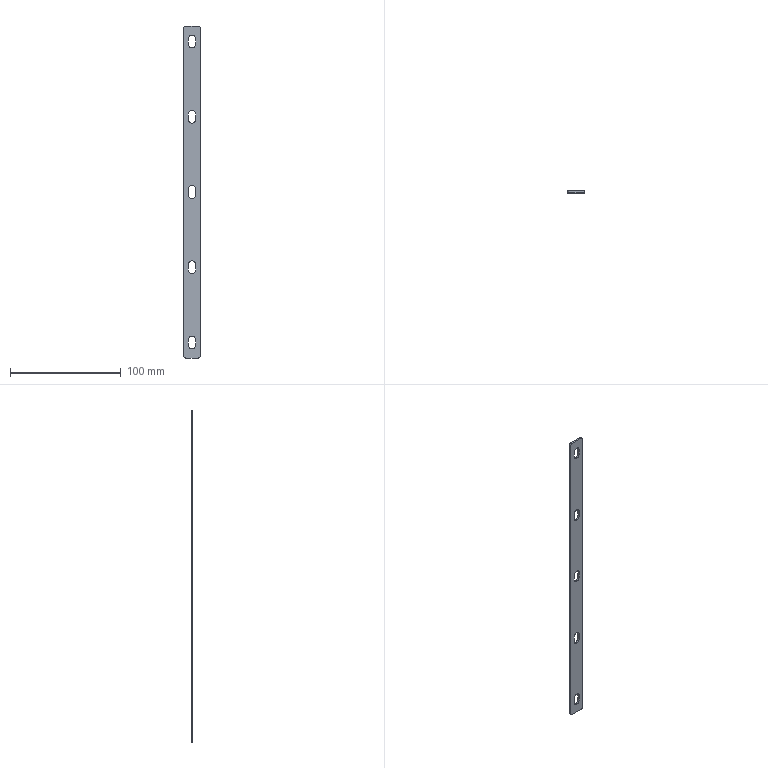Part | 1 solid | 35 faces | box 15 x 1.5 x 300 mm | volume 6252 mm3 | cylinder 19 | plane 16 | commonest cylinder face diameters 6.5 x15 4 x4
STEP:
#1=CARTESIAN_POINT('',(0.,-1.5,141.75));
#2=VERTEX_POINT('',#1);
#3=CARTESIAN_POINT('',(3.25,-1.5,138.5));
#4=VERTEX_POINT('',#3);
#5=CARTESIAN_POINT('',(0.,-1.5,138.5));
#6=DIRECTION('',(0.,1.,0.));
#7=DIRECTION('',(0.,0.,1.));
#8=AXIS2_PLACEMENT_3D('',#5,#6,#7);
#9=CIRCLE('',#8,3.25);
#10=EDGE_CURVE('',#2,#4,#9,.T.);
#11=ORIENTED_EDGE('',*,*,#10,.F.);
#12=CARTESIAN_POINT('',(0.,0.,141.75));
#13=VERTEX_POINT('',#12);
#14=CARTESIAN_POINT('',(0.,-1.5,141.75));
#15=DIRECTION('',(0.,1.,0.));
#16=VECTOR('',#15,1000.);
#17=LINE('',#14,#16);
#18=EDGE_CURVE('',#2,#13,#17,.T.);
#19=ORIENTED_EDGE('',*,*,#18,.T.);
#20=CARTESIAN_POINT('',(3.25,0.,138.5));
#21=VERTEX_POINT('',#20);
#22=CARTESIAN_POINT('',(0.,0.,138.5));
#23=DIRECTION('',(0.,1.,0.));
#24=DIRECTION('',(0.,0.,1.));
#25=AXIS2_PLACEMENT_3D('',#22,#23,#24);
#26=CIRCLE('',#25,3.25);
#27=EDGE_CURVE('',#13,#21,#26,.T.);
#28=ORIENTED_EDGE('',*,*,#27,.T.);
#29=CARTESIAN_POINT('',(3.25,-1.5,138.5));
#30=DIRECTION('',(0.,1.,0.));
#31=VECTOR('',#30,1000.);
#32=LINE('',#29,#31);
#33=EDGE_CURVE('',#4,#21,#32,.T.);
#34=ORIENTED_EDGE('',*,*,#33,.F.);
#35=EDGE_LOOP('',(#11,#19,#28,#34));
#36=FACE_OUTER_BOUND('',#35,.T.);
#37=CARTESIAN_POINT('',(0.,-1.5,138.5));
#38=DIRECTION('',(0.,1.,0.));
#39=DIRECTION('',(0.,0.,1.));
#40=AXIS2_PLACEMENT_3D('',#37,#38,#39);
#41=CYLINDRICAL_SURFACE('',#40,3.25);
#42=ADVANCED_FACE('',(#36),#41,.F.);
#43=CARTESIAN_POINT('',(0.,-1.5,73.75));
#44=VERTEX_POINT('',#43);
#45=CARTESIAN_POINT('',(3.25,-1.5,70.5));
#46=VERTEX_POINT('',#45);
#47=CARTESIAN_POINT('',(0.,-1.5,70.5));
#48=DIRECTION('',(0.,1.,0.));
#49=DIRECTION('',(0.,0.,1.));
#50=AXIS2_PLACEMENT_3D('',#47,#48,#49);
#51=CIRCLE('',#50,3.25);
#52=EDGE_CURVE('',#44,#46,#51,.T.);
#53=ORIENTED_EDGE('',*,*,#52,.F.);
#54=CARTESIAN_POINT('',(0.,0.,73.75));
#55=VERTEX_POINT('',#54);
#56=CARTESIAN_POINT('',(0.,-1.5,73.75));
#57=DIRECTION('',(0.,1.,0.));
#58=VECTOR('',#57,1000.);
#59=LINE('',#56,#58);
#60=EDGE_CURVE('',#44,#55,#59,.T.);
#61=ORIENTED_EDGE('',*,*,#60,.T.);
#62=CARTESIAN_POINT('',(3.25,0.,70.5));
#63=VERTEX_POINT('',#62);
#64=CARTESIAN_POINT('',(0.,0.,70.5));
#65=DIRECTION('',(0.,1.,0.));
#66=DIRECTION('',(0.,0.,1.));
#67=AXIS2_PLACEMENT_3D('',#64,#65,#66);
#68=CIRCLE('',#67,3.25);
#69=EDGE_CURVE('',#55,#63,#68,.T.);
#70=ORIENTED_EDGE('',*,*,#69,.T.);
#71=CARTESIAN_POINT('',(3.25,-1.5,70.5));
#72=DIRECTION('',(0.,1.,0.));
#73=VECTOR('',#72,1000.);
#74=LINE('',#71,#73);
#75=EDGE_CURVE('',#46,#63,#74,.T.);
#76=ORIENTED_EDGE('',*,*,#75,.F.);
#77=EDGE_LOOP('',(#53,#61,#70,#76));
#78=FACE_OUTER_BOUND('',#77,.T.);
#79=CARTESIAN_POINT('',(0.,-1.5,70.5));
#80=DIRECTION('',(0.,1.,0.));
#81=DIRECTION('',(0.,0.,1.));
#82=AXIS2_PLACEMENT_3D('',#79,#80,#81);
#83=CYLINDRICAL_SURFACE('',#82,3.25);
#84=ADVANCED_FACE('',(#78),#83,.F.);
#85=CARTESIAN_POINT('',(0.,-1.5,5.75));
#86=VERTEX_POINT('',#85);
#87=CARTESIAN_POINT('',(3.25,-1.5,2.5));
#88=VERTEX_POINT('',#87);
#89=CARTESIAN_POINT('',(0.,-1.5,2.5));
#90=DIRECTION('',(0.,1.,0.));
#91=DIRECTION('',(0.,0.,1.));
#92=AXIS2_PLACEMENT_3D('',#89,#90,#91);
#93=CIRCLE('',#92,3.25);
#94=EDGE_CURVE('',#86,#88,#93,.T.);
#95=ORIENTED_EDGE('',*,*,#94,.F.);
#96=CARTESIAN_POINT('',(0.,0.,5.75));
#97=VERTEX_POINT('',#96);
#98=CARTESIAN_POINT('',(0.,-1.5,5.75));
#99=DIRECTION('',(0.,1.,0.));
#100=VECTOR('',#99,1000.);
#101=LINE('',#98,#100);
#102=EDGE_CURVE('',#86,#97,#101,.T.);
#103=ORIENTED_EDGE('',*,*,#102,.T.);
#104=CARTESIAN_POINT('',(3.25,0.,2.5));
#105=VERTEX_POINT('',#104);
#106=CARTESIAN_POINT('',(0.,0.,2.5));
#107=DIRECTION('',(0.,1.,0.));
#108=DIRECTION('',(0.,0.,1.));
#109=AXIS2_PLACEMENT_3D('',#106,#107,#108);
#110=CIRCLE('',#109,3.25);
#111=EDGE_CURVE('',#97,#105,#110,.T.);
#112=ORIENTED_EDGE('',*,*,#111,.T.);
#113=CARTESIAN_POINT('',(3.25,-1.5,2.5));
#114=DIRECTION('',(0.,1.,0.));
#115=VECTOR('',#114,1000.);
#116=LINE('',#113,#115);
#117=EDGE_CURVE('',#88,#105,#116,.T.);
#118=ORIENTED_EDGE('',*,*,#117,.F.);
#119=EDGE_LOOP('',(#95,#103,#112,#118));
#120=FACE_OUTER_BOUND('',#119,.T.);
#121=CARTESIAN_POINT('',(0.,-1.5,2.5));
#122=DIRECTION('',(0.,1.,0.));
#123=DIRECTION('',(0.,0.,1.));
#124=AXIS2_PLACEMENT_3D('',#121,#122,#123);
#125=CYLINDRICAL_SURFACE('',#124,3.25);
#126=ADVANCED_FACE('',(#120),#125,.F.);
#127=CARTESIAN_POINT('',(0.,-1.5,-62.25));
#128=VERTEX_POINT('',#127);
#129=CARTESIAN_POINT('',(3.25,-1.5,-65.5));
#130=VERTEX_POINT('',#129);
#131=CARTESIAN_POINT('',(0.,-1.5,-65.5));
#132=DIRECTION('',(0.,1.,0.));
#133=DIRECTION('',(0.,0.,1.));
#134=AXIS2_PLACEMENT_3D('',#131,#132,#133);
#135=CIRCLE('',#134,3.25);
#136=EDGE_CURVE('',#128,#130,#135,.T.);
#137=ORIENTED_EDGE('',*,*,#136,.F.);
#138=CARTESIAN_POINT('',(0.,0.,-62.25));
#139=VERTEX_POINT('',#138);
#140=CARTESIAN_POINT('',(0.,-1.5,-62.25));
#141=DIRECTION('',(0.,1.,0.));
#142=VECTOR('',#141,1000.);
#143=LINE('',#140,#142);
#144=EDGE_CURVE('',#128,#139,#143,.T.);
#145=ORIENTED_EDGE('',*,*,#144,.T.);
#146=CARTESIAN_POINT('',(3.25,0.,-65.5));
#147=VERTEX_POINT('',#146);
#148=CARTESIAN_POINT('',(0.,0.,-65.5));
#149=DIRECTION('',(0.,1.,0.));
#150=DIRECTION('',(0.,0.,1.));
#151=AXIS2_PLACEMENT_3D('',#148,#149,#150);
#152=CIRCLE('',#151,3.25);
#153=EDGE_CURVE('',#139,#147,#152,.T.);
#154=ORIENTED_EDGE('',*,*,#153,.T.);
#155=CARTESIAN_POINT('',(3.25,-1.5,-65.5));
#156=DIRECTION('',(0.,1.,0.));
#157=VECTOR('',#156,1000.);
#158=LINE('',#155,#157);
#159=EDGE_CURVE('',#130,#147,#158,.T.);
#160=ORIENTED_EDGE('',*,*,#159,.F.);
#161=EDGE_LOOP('',(#137,#145,#154,#160));
#162=FACE_OUTER_BOUND('',#161,.T.);
#163=CARTESIAN_POINT('',(0.,-1.5,-65.5));
#164=DIRECTION('',(0.,1.,0.));
#165=DIRECTION('',(0.,0.,1.));
#166=AXIS2_PLACEMENT_3D('',#163,#164,#165);
#167=CYLINDRICAL_SURFACE('',#166,3.25);
#168=ADVANCED_FACE('',(#162),#167,.F.);
#169=CARTESIAN_POINT('',(0.,-1.5,-130.25));
#170=VERTEX_POINT('',#169);
#171=CARTESIAN_POINT('',(3.25,-1.5,-133.5));
#172=VERTEX_POINT('',#171);
#173=CARTESIAN_POINT('',(0.,-1.5,-133.5));
#174=DIRECTION('',(0.,1.,0.));
#175=DIRECTION('',(0.,0.,1.));
#176=AXIS2_PLACEMENT_3D('',#173,#174,#175);
#177=CIRCLE('',#176,3.25);
#178=EDGE_CURVE('',#170,#172,#177,.T.);
#179=ORIENTED_EDGE('',*,*,#178,.F.);
#180=CARTESIAN_POINT('',(0.,0.,-130.25));
#181=VERTEX_POINT('',#180);
#182=CARTESIAN_POINT('',(0.,-1.5,-130.25));
#183=DIRECTION('',(0.,1.,0.));
#184=VECTOR('',#183,1000.);
#185=LINE('',#182,#184);
#186=EDGE_CURVE('',#170,#181,#185,.T.);
#187=ORIENTED_EDGE('',*,*,#186,.T.);
#188=CARTESIAN_POINT('',(3.25,0.,-133.5));
#189=VERTEX_POINT('',#188);
#190=CARTESIAN_POINT('',(0.,0.,-133.5));
#191=DIRECTION('',(0.,1.,0.));
#192=DIRECTION('',(0.,0.,1.));
#193=AXIS2_PLACEMENT_3D('',#190,#191,#192);
#194=CIRCLE('',#193,3.25);
#195=EDGE_CURVE('',#181,#189,#194,.T.);
#196=ORIENTED_EDGE('',*,*,#195,.T.);
#197=CARTESIAN_POINT('',(3.25,-1.5,-133.5));
#198=DIRECTION('',(0.,1.,0.));
#199=VECTOR('',#198,1000.);
#200=LINE('',#197,#199);
#201=EDGE_CURVE('',#172,#189,#200,.T.);
#202=ORIENTED_EDGE('',*,*,#201,.F.);
#203=EDGE_LOOP('',(#179,#187,#196,#202));
#204=FACE_OUTER_BOUND('',#203,.T.);
#205=CARTESIAN_POINT('',(0.,-1.5,-133.5));
#206=DIRECTION('',(0.,1.,0.));
#207=DIRECTION('',(0.,0.,1.));
#208=AXIS2_PLACEMENT_3D('',#205,#206,#207);
#209=CYLINDRICAL_SURFACE('',#208,3.25);
#210=ADVANCED_FACE('',(#204),#209,.F.);
#211=CARTESIAN_POINT('',(7.5,0.,148.));
#212=VERTEX_POINT('',#211);
#213=CARTESIAN_POINT('',(7.5,0.,-148.));
#214=VERTEX_POINT('',#213);
#215=CARTESIAN_POINT('',(7.5,0.,150.));
#216=DIRECTION('',(0.,0.,-1.));
#217=VECTOR('',#216,1000.);
#218=LINE('',#215,#217);
#219=EDGE_CURVE('',#212,#214,#218,.T.);
#220=ORIENTED_EDGE('',*,*,#219,.F.);
#221=CARTESIAN_POINT('',(7.5,-1.5,148.));
#222=VERTEX_POINT('',#221);
#223=CARTESIAN_POINT('',(7.5,-1.5,148.));
#224=DIRECTION('',(0.,-1.,0.));
#225=VECTOR('',#224,1000.);
#226=LINE('',#223,#225);
#227=EDGE_CURVE('',#212,#222,#226,.T.);
#228=ORIENTED_EDGE('',*,*,#227,.T.);
#229=CARTESIAN_POINT('',(7.5,-1.5,-148.));
#230=VERTEX_POINT('',#229);
#231=CARTESIAN_POINT('',(7.5,-1.5,150.));
#232=DIRECTION('',(0.,0.,-1.));
#233=VECTOR('',#232,1000.);
#234=LINE('',#231,#233);
#235=EDGE_CURVE('',#222,#230,#234,.T.);
#236=ORIENTED_EDGE('',*,*,#235,.T.);
#237=CARTESIAN_POINT('',(7.5,-1.5,-148.));
#238=DIRECTION('',(0.,1.,0.));
#239=VECTOR('',#238,1000.);
#240=LINE('',#237,#239);
#241=EDGE_CURVE('',#230,#214,#240,.T.);
#242=ORIENTED_EDGE('',*,*,#241,.T.);
#243=EDGE_LOOP('',(#220,#228,#236,#242));
#244=FACE_OUTER_BOUND('',#243,.T.);
#245=CARTESIAN_POINT('',(7.5,-1.5,150.));
#246=DIRECTION('',(1.,0.,0.));
#247=DIRECTION('',(0.,0.,-1.));
#248=AXIS2_PLACEMENT_3D('',#245,#246,#247);
#249=PLANE('',#248);
#250=ADVANCED_FACE('',(#244),#249,.T.);
#251=CARTESIAN_POINT('',(-5.5,-1.5,150.));
#252=VERTEX_POINT('',#251);
#253=CARTESIAN_POINT('',(5.5,-1.5,150.));
#254=VERTEX_POINT('',#253);
#255=CARTESIAN_POINT('',(-7.5,-1.5,150.));
#256=DIRECTION('',(1.,0.,0.));
#257=VECTOR('',#256,1000.);
#258=LINE('',#255,#257);
#259=EDGE_CURVE('',#252,#254,#258,.T.);
#260=ORIENTED_EDGE('',*,*,#259,.T.);
#261=CARTESIAN_POINT('',(5.5,0.,150.));
#262=VERTEX_POINT('',#261);
#263=CARTESIAN_POINT('',(5.5,-1.5,150.));
#264=DIRECTION('',(0.,1.,0.));
#265=VECTOR('',#264,1000.);
#266=LINE('',#263,#265);
#267=EDGE_CURVE('',#254,#262,#266,.T.);
#268=ORIENTED_EDGE('',*,*,#267,.T.);
#269=CARTESIAN_POINT('',(-5.5,0.,150.));
#270=VERTEX_POINT('',#269);
#271=CARTESIAN_POINT('',(-7.5,0.,150.));
#272=DIRECTION('',(1.,0.,0.));
#273=VECTOR('',#272,1000.);
#274=LINE('',#271,#273);
#275=EDGE_CURVE('',#270,#262,#274,.T.);
#276=ORIENTED_EDGE('',*,*,#275,.F.);
#277=CARTESIAN_POINT('',(-5.5,-1.5,150.));
#278=DIRECTION('',(0.,-1.,0.));
#279=VECTOR('',#278,1000.);
#280=LINE('',#277,#279);
#281=EDGE_CURVE('',#270,#252,#280,.T.);
#282=ORIENTED_EDGE('',*,*,#281,.T.);
#283=EDGE_LOOP('',(#260,#268,#276,#282));
#284=FACE_OUTER_BOUND('',#283,.T.);
#285=CARTESIAN_POINT('',(-7.5,-1.5,150.));
#286=DIRECTION('',(0.,0.,1.));
#287=DIRECTION('',(1.,0.,0.));
#288=AXIS2_PLACEMENT_3D('',#285,#286,#287);
#289=PLANE('',#288);
#290=ADVANCED_FACE('',(#284),#289,.T.);
#291=CARTESIAN_POINT('',(-7.5,-1.5,-148.));
#292=VERTEX_POINT('',#291);
#293=CARTESIAN_POINT('',(-7.5,-1.5,148.));
#294=VERTEX_POINT('',#293);
#295=CARTESIAN_POINT('',(-7.5,-1.5,150.));
#296=DIRECTION('',(0.,0.,1.));
#297=VECTOR('',#296,1000.);
#298=LINE('',#295,#297);
#299=EDGE_CURVE('',#292,#294,#298,.T.);
#300=ORIENTED_EDGE('',*,*,#299,.T.);
#301=CARTESIAN_POINT('',(-7.5,0.,148.));
#302=VERTEX_POINT('',#301);
#303=CARTESIAN_POINT('',(-7.5,-1.5,148.));
#304=DIRECTION('',(0.,1.,0.));
#305=VECTOR('',#304,1000.);
#306=LINE('',#303,#305);
#307=EDGE_CURVE('',#294,#302,#306,.T.);
#308=ORIENTED_EDGE('',*,*,#307,.T.);
#309=CARTESIAN_POINT('',(-7.5,0.,-148.));
#310=VERTEX_POINT('',#309);
#311=CARTESIAN_POINT('',(-7.5,0.,150.));
#312=DIRECTION('',(0.,0.,1.));
#313=VECTOR('',#312,1000.);
#314=LINE('',#311,#313);
#315=EDGE_CURVE('',#310,#302,#314,.T.);
#316=ORIENTED_EDGE('',*,*,#315,.F.);
#317=CARTESIAN_POINT('',(-7.5,-1.5,-148.));
#318=DIRECTION('',(0.,-1.,0.));
#319=VECTOR('',#318,1000.);
#320=LINE('',#317,#319);
#321=EDGE_CURVE('',#310,#292,#320,.T.);
#322=ORIENTED_EDGE('',*,*,#321,.T.);
#323=EDGE_LOOP('',(#300,#308,#316,#322));
#324=FACE_OUTER_BOUND('',#323,.T.);
#325=CARTESIAN_POINT('',(-7.5,-1.5,150.));
#326=DIRECTION('',(-1.,0.,0.));
#327=DIRECTION('',(0.,0.,1.));
#328=AXIS2_PLACEMENT_3D('',#325,#326,#327);
#329=PLANE('',#328);
#330=ADVANCED_FACE('',(#324),#329,.T.);
#331=CARTESIAN_POINT('',(5.5,-1.5,-150.));
#332=VERTEX_POINT('',#331);
#333=CARTESIAN_POINT('',(-5.5,-1.5,-150.));
#334=VERTEX_POINT('',#333);
#335=CARTESIAN_POINT('',(-7.5,-1.5,-150.));
#336=DIRECTION('',(-1.,0.,0.));
#337=VECTOR('',#336,1000.);
#338=LINE('',#335,#337);
#339=EDGE_CURVE('',#332,#334,#338,.T.);
#340=ORIENTED_EDGE('',*,*,#339,.T.);
#341=CARTESIAN_POINT('',(-5.5,0.,-150.));
#342=VERTEX_POINT('',#341);
#343=CARTESIAN_POINT('',(-5.5,-1.5,-150.));
#344=DIRECTION('',(0.,1.,0.));
#345=VECTOR('',#344,1000.);
#346=LINE('',#343,#345);
#347=EDGE_CURVE('',#334,#342,#346,.T.);
#348=ORIENTED_EDGE('',*,*,#347,.T.);
#349=CARTESIAN_POINT('',(5.5,0.,-150.));
#350=VERTEX_POINT('',#349);
#351=CARTESIAN_POINT('',(-7.5,0.,-150.));
#352=DIRECTION('',(-1.,0.,0.));
#353=VECTOR('',#352,1000.);
#354=LINE('',#351,#353);
#355=EDGE_CURVE('',#350,#342,#354,.T.);
#356=ORIENTED_EDGE('',*,*,#355,.F.);
#357=CARTESIAN_POINT('',(5.5,-1.5,-150.));
#358=DIRECTION('',(0.,-1.,0.));
#359=VECTOR('',#358,1000.);
#360=LINE('',#357,#359);
#361=EDGE_CURVE('',#350,#332,#360,.T.);
#362=ORIENTED_EDGE('',*,*,#361,.T.);
#363=EDGE_LOOP('',(#340,#348,#356,#362));
#364=FACE_OUTER_BOUND('',#363,.T.);
#365=CARTESIAN_POINT('',(-7.5,-1.5,-150.));
#366=DIRECTION('',(0.,0.,-1.));
#367=DIRECTION('',(-1.,0.,0.));
#368=AXIS2_PLACEMENT_3D('',#365,#366,#367);
#369=PLANE('',#368);
#370=ADVANCED_FACE('',(#364),#369,.T.);
#371=CARTESIAN_POINT('',(-3.25,-1.5,138.5));
#372=VERTEX_POINT('',#371);
#373=CARTESIAN_POINT('',(0.,-1.5,138.5));
#374=DIRECTION('',(0.,1.,0.));
#375=DIRECTION('',(0.,0.,1.));
#376=AXIS2_PLACEMENT_3D('',#373,#374,#375);
#377=CIRCLE('',#376,3.25);
#378=EDGE_CURVE('',#372,#2,#377,.T.);
#379=ORIENTED_EDGE('',*,*,#378,.T.);
#380=ORIENTED_EDGE('',*,*,#10,.T.);
#381=CARTESIAN_POINT('',(3.25,-1.5,133.5));
#382=VERTEX_POINT('',#381);
#383=CARTESIAN_POINT('',(3.25,-1.5,138.5));
#384=DIRECTION('',(0.,0.,-1.));
#385=VECTOR('',#384,1000.);
#386=LINE('',#383,#385);
#387=EDGE_CURVE('',#4,#382,#386,.T.);
#388=ORIENTED_EDGE('',*,*,#387,.T.);
#389=CARTESIAN_POINT('',(-3.25,-1.5,133.5));
#390=VERTEX_POINT('',#389);
#391=CARTESIAN_POINT('',(0.,-1.5,133.5));
#392=DIRECTION('',(0.,1.,0.));
#393=DIRECTION('',(0.,0.,1.));
#394=AXIS2_PLACEMENT_3D('',#391,#392,#393);
#395=CIRCLE('',#394,3.25);
#396=EDGE_CURVE('',#382,#390,#395,.T.);
#397=ORIENTED_EDGE('',*,*,#396,.T.);
#398=CARTESIAN_POINT('',(-3.25,-1.5,138.5));
#399=DIRECTION('',(0.,0.,1.));
#400=VECTOR('',#399,1000.);
#401=LINE('',#398,#400);
#402=EDGE_CURVE('',#390,#372,#401,.T.);
#403=ORIENTED_EDGE('',*,*,#402,.T.);
#404=EDGE_LOOP('',(#379,#380,#388,#397,#403));
#405=FACE_BOUND('',#404,.T.);
#406=CARTESIAN_POINT('',(-3.25,-1.5,70.5));
#407=VERTEX_POINT('',#406);
#408=CARTESIAN_POINT('',(0.,-1.5,70.5));
#409=DIRECTION('',(0.,1.,0.));
#410=DIRECTION('',(0.,0.,1.));
#411=AXIS2_PLACEMENT_3D('',#408,#409,#410);
#412=CIRCLE('',#411,3.25);
#413=EDGE_CURVE('',#407,#44,#412,.T.);
#414=ORIENTED_EDGE('',*,*,#413,.T.);
#415=ORIENTED_EDGE('',*,*,#52,.T.);
#416=CARTESIAN_POINT('',(3.25,-1.5,65.5));
#417=VERTEX_POINT('',#416);
#418=CARTESIAN_POINT('',(3.25,-1.5,70.5));
#419=DIRECTION('',(0.,0.,-1.));
#420=VECTOR('',#419,1000.);
#421=LINE('',#418,#420);
#422=EDGE_CURVE('',#46,#417,#421,.T.);
#423=ORIENTED_EDGE('',*,*,#422,.T.);
#424=CARTESIAN_POINT('',(-3.25,-1.5,65.5));
#425=VERTEX_POINT('',#424);
#426=CARTESIAN_POINT('',(0.,-1.5,65.5));
#427=DIRECTION('',(0.,1.,0.));
#428=DIRECTION('',(0.,0.,1.));
#429=AXIS2_PLACEMENT_3D('',#426,#427,#428);
#430=CIRCLE('',#429,3.25);
#431=EDGE_CURVE('',#417,#425,#430,.T.);
#432=ORIENTED_EDGE('',*,*,#431,.T.);
#433=CARTESIAN_POINT('',(-3.25,-1.5,70.5));
#434=DIRECTION('',(0.,0.,1.));
#435=VECTOR('',#434,1000.);
#436=LINE('',#433,#435);
#437=EDGE_CURVE('',#425,#407,#436,.T.);
#438=ORIENTED_EDGE('',*,*,#437,.T.);
#439=EDGE_LOOP('',(#414,#415,#423,#432,#438));
#440=FACE_BOUND('',#439,.T.);
#441=CARTESIAN_POINT('',(-3.25,-1.5,2.5));
#442=VERTEX_POINT('',#441);
#443=CARTESIAN_POINT('',(0.,-1.5,2.5));
#444=DIRECTION('',(0.,1.,0.));
#445=DIRECTION('',(0.,0.,1.));
#446=AXIS2_PLACEMENT_3D('',#443,#444,#445);
#447=CIRCLE('',#446,3.25);
#448=EDGE_CURVE('',#442,#86,#447,.T.);
#449=ORIENTED_EDGE('',*,*,#448,.T.);
#450=ORIENTED_EDGE('',*,*,#94,.T.);
#451=CARTESIAN_POINT('',(3.25,-1.5,-2.5));
#452=VERTEX_POINT('',#451);
#453=CARTESIAN_POINT('',(3.25,-1.5,2.5));
#454=DIRECTION('',(0.,0.,-1.));
#455=VECTOR('',#454,1000.);
#456=LINE('',#453,#455);
#457=EDGE_CURVE('',#88,#452,#456,.T.);
#458=ORIENTED_EDGE('',*,*,#457,.T.);
#459=CARTESIAN_POINT('',(-3.25,-1.5,-2.5));
#460=VERTEX_POINT('',#459);
#461=CARTESIAN_POINT('',(0.,-1.5,-2.5));
#462=DIRECTION('',(0.,1.,0.));
#463=DIRECTION('',(0.,0.,1.));
#464=AXIS2_PLACEMENT_3D('',#461,#462,#463);
#465=CIRCLE('',#464,3.25);
#466=EDGE_CURVE('',#452,#460,#465,.T.);
#467=ORIENTED_EDGE('',*,*,#466,.T.);
#468=CARTESIAN_POINT('',(-3.25,-1.5,2.5));
#469=DIRECTION('',(0.,0.,1.));
#470=VECTOR('',#469,1000.);
#471=LINE('',#468,#470);
#472=EDGE_CURVE('',#460,#442,#471,.T.);
#473=ORIENTED_EDGE('',*,*,#472,.T.);
#474=EDGE_LOOP('',(#449,#450,#458,#467,#473));
#475=FACE_BOUND('',#474,.T.);
#476=CARTESIAN_POINT('',(-3.25,-1.5,-65.5));
#477=VERTEX_POINT('',#476);
#478=CARTESIAN_POINT('',(0.,-1.5,-65.5));
#479=DIRECTION('',(0.,1.,0.));
#480=DIRECTION('',(0.,0.,1.));
#481=AXIS2_PLACEMENT_3D('',#478,#479,#480);
#482=CIRCLE('',#481,3.25);
#483=EDGE_CURVE('',#477,#128,#482,.T.);
#484=ORIENTED_EDGE('',*,*,#483,.T.);
#485=ORIENTED_EDGE('',*,*,#136,.T.);
#486=CARTESIAN_POINT('',(3.25,-1.5,-70.5));
#487=VERTEX_POINT('',#486);
#488=CARTESIAN_POINT('',(3.25,-1.5,-65.5));
#489=DIRECTION('',(0.,0.,-1.));
#490=VECTOR('',#489,1000.);
#491=LINE('',#488,#490);
#492=EDGE_CURVE('',#130,#487,#491,.T.);
#493=ORIENTED_EDGE('',*,*,#492,.T.);
#494=CARTESIAN_POINT('',(-3.25,-1.5,-70.5));
#495=VERTEX_POINT('',#494);
#496=CARTESIAN_POINT('',(0.,-1.5,-70.5));
#497=DIRECTION('',(0.,1.,0.));
#498=DIRECTION('',(0.,0.,1.));
#499=AXIS2_PLACEMENT_3D('',#496,#497,#498);
#500=CIRCLE('',#499,3.25);
#501=EDGE_CURVE('',#487,#495,#500,.T.);
#502=ORIENTED_EDGE('',*,*,#501,.T.);
#503=CARTESIAN_POINT('',(-3.25,-1.5,-65.5));
#504=DIRECTION('',(0.,0.,1.));
#505=VECTOR('',#504,1000.);
#506=LINE('',#503,#505);
#507=EDGE_CURVE('',#495,#477,#506,.T.);
#508=ORIENTED_EDGE('',*,*,#507,.T.);
#509=EDGE_LOOP('',(#484,#485,#493,#502,#508));
#510=FACE_BOUND('',#509,.T.);
#511=CARTESIAN_POINT('',(-3.25,-1.5,-133.5));
#512=VERTEX_POINT('',#511);
#513=CARTESIAN_POINT('',(0.,-1.5,-133.5));
#514=DIRECTION('',(0.,1.,0.));
#515=DIRECTION('',(0.,0.,1.));
#516=AXIS2_PLACEMENT_3D('',#513,#514,#515);
#517=CIRCLE('',#516,3.25);
#518=EDGE_CURVE('',#512,#170,#517,.T.);
#519=ORIENTED_EDGE('',*,*,#518,.T.);
#520=ORIENTED_EDGE('',*,*,#178,.T.);
#521=CARTESIAN_POINT('',(3.25,-1.5,-138.5));
#522=VERTEX_POINT('',#521);
#523=CARTESIAN_POINT('',(3.25,-1.5,-133.5));
#524=DIRECTION('',(0.,0.,-1.));
#525=VECTOR('',#524,1000.);
#526=LINE('',#523,#525);
#527=EDGE_CURVE('',#172,#522,#526,.T.);
#528=ORIENTED_EDGE('',*,*,#527,.T.);
#529=CARTESIAN_POINT('',(-3.25,-1.5,-138.5));
#530=VERTEX_POINT('',#529);
#531=CARTESIAN_POINT('',(0.,-1.5,-138.5));
#532=DIRECTION('',(0.,1.,0.));
#533=DIRECTION('',(0.,0.,1.));
#534=AXIS2_PLACEMENT_3D('',#531,#532,#533);
#535=CIRCLE('',#534,3.25);
#536=EDGE_CURVE('',#522,#530,#535,.T.);
#537=ORIENTED_EDGE('',*,*,#536,.T.);
#538=CARTESIAN_POINT('',(-3.25,-1.5,-133.5));
#539=DIRECTION('',(0.,0.,1.));
#540=VECTOR('',#539,1000.);
#541=LINE('',#538,#540);
#542=EDGE_CURVE('',#530,#512,#541,.T.);
#543=ORIENTED_EDGE('',*,*,#542,.T.);
#544=EDGE_LOOP('',(#519,#520,#528,#537,#543));
#545=FACE_BOUND('',#544,.T.);
#546=ORIENTED_EDGE('',*,*,#235,.F.);
#547=CARTESIAN_POINT('',(5.5,-1.5,148.));
#548=DIRECTION('',(0.,-1.,0.));
#549=DIRECTION('',(0.,0.,-1.));
#550=AXIS2_PLACEMENT_3D('',#547,#548,#549);
#551=CIRCLE('',#550,2.);
#552=EDGE_CURVE('',#222,#254,#551,.T.);
#553=ORIENTED_EDGE('',*,*,#552,.T.);
#554=ORIENTED_EDGE('',*,*,#259,.F.);
#555=CARTESIAN_POINT('',(-5.5,-1.5,148.));
#556=DIRECTION('',(0.,-1.,0.));
#557=DIRECTION('',(0.,0.,-1.));
#558=AXIS2_PLACEMENT_3D('',#555,#556,#557);
#559=CIRCLE('',#558,2.);
#560=EDGE_CURVE('',#252,#294,#559,.T.);
#561=ORIENTED_EDGE('',*,*,#560,.T.);
#562=ORIENTED_EDGE('',*,*,#299,.F.);
#563=CARTESIAN_POINT('',(-5.5,-1.5,-148.));
#564=DIRECTION('',(0.,-1.,0.));
#565=DIRECTION('',(0.,0.,-1.));
#566=AXIS2_PLACEMENT_3D('',#563,#564,#565);
#567=CIRCLE('',#566,2.);
#568=EDGE_CURVE('',#292,#334,#567,.T.);
#569=ORIENTED_EDGE('',*,*,#568,.T.);
#570=ORIENTED_EDGE('',*,*,#339,.F.);
#571=CARTESIAN_POINT('',(5.5,-1.5,-148.));
#572=DIRECTION('',(0.,-1.,0.));
#573=DIRECTION('',(0.,0.,-1.));
#574=AXIS2_PLACEMENT_3D('',#571,#572,#573);
#575=CIRCLE('',#574,2.);
#576=EDGE_CURVE('',#332,#230,#575,.T.);
#577=ORIENTED_EDGE('',*,*,#576,.T.);
#578=EDGE_LOOP('',(#546,#553,#554,#561,#562,#569,#570,#577));
#579=FACE_OUTER_BOUND('',#578,.T.);
#580=CARTESIAN_POINT('',(0.,-1.5,0.));
#581=DIRECTION('',(0.,-1.,0.));
#582=DIRECTION('',(0.,0.,-1.));
#583=AXIS2_PLACEMENT_3D('',#580,#581,#582);
#584=PLANE('',#583);
#585=ADVANCED_FACE('',(#405,#440,#475,#510,#545,#579),#584,.T.);
#586=CARTESIAN_POINT('',(3.25,0.,133.5));
#587=VERTEX_POINT('',#586);
#588=CARTESIAN_POINT('',(3.25,0.,138.5));
#589=DIRECTION('',(0.,0.,-1.));
#590=VECTOR('',#589,1000.);
#591=LINE('',#588,#590);
#592=EDGE_CURVE('',#21,#587,#591,.T.);
#593=ORIENTED_EDGE('',*,*,#592,.F.);
#594=ORIENTED_EDGE('',*,*,#27,.F.);
#595=CARTESIAN_POINT('',(-3.25,0.,138.5));
#596=VERTEX_POINT('',#595);
#597=CARTESIAN_POINT('',(0.,0.,138.5));
#598=DIRECTION('',(0.,1.,0.));
#599=DIRECTION('',(0.,0.,1.));
#600=AXIS2_PLACEMENT_3D('',#597,#598,#599);
#601=CIRCLE('',#600,3.25);
#602=EDGE_CURVE('',#596,#13,#601,.T.);
#603=ORIENTED_EDGE('',*,*,#602,.F.);
#604=CARTESIAN_POINT('',(-3.25,0.,133.5));
#605=VERTEX_POINT('',#604);
#606=CARTESIAN_POINT('',(-3.25,0.,138.5));
#607=DIRECTION('',(0.,0.,1.));
#608=VECTOR('',#607,1000.);
#609=LINE('',#606,#608);
#610=EDGE_CURVE('',#605,#596,#609,.T.);
#611=ORIENTED_EDGE('',*,*,#610,.F.);
#612=CARTESIAN_POINT('',(0.,0.,133.5));
#613=DIRECTION('',(0.,1.,0.));
#614=DIRECTION('',(0.,0.,1.));
#615=AXIS2_PLACEMENT_3D('',#612,#613,#614);
#616=CIRCLE('',#615,3.25);
#617=EDGE_CURVE('',#587,#605,#616,.T.);
#618=ORIENTED_EDGE('',*,*,#617,.F.);
#619=EDGE_LOOP('',(#593,#594,#603,#611,#618));
#620=FACE_BOUND('',#619,.T.);
#621=CARTESIAN_POINT('',(3.25,0.,65.5));
#622=VERTEX_POINT('',#621);
#623=CARTESIAN_POINT('',(3.25,0.,70.5));
#624=DIRECTION('',(0.,0.,-1.));
#625=VECTOR('',#624,1000.);
#626=LINE('',#623,#625);
#627=EDGE_CURVE('',#63,#622,#626,.T.);
#628=ORIENTED_EDGE('',*,*,#627,.F.);
#629=ORIENTED_EDGE('',*,*,#69,.F.);
#630=CARTESIAN_POINT('',(-3.25,0.,70.5));
#631=VERTEX_POINT('',#630);
#632=CARTESIAN_POINT('',(0.,0.,70.5));
#633=DIRECTION('',(0.,1.,0.));
#634=DIRECTION('',(0.,0.,1.));
#635=AXIS2_PLACEMENT_3D('',#632,#633,#634);
#636=CIRCLE('',#635,3.25);
#637=EDGE_CURVE('',#631,#55,#636,.T.);
#638=ORIENTED_EDGE('',*,*,#637,.F.);
#639=CARTESIAN_POINT('',(-3.25,0.,65.5));
#640=VERTEX_POINT('',#639);
#641=CARTESIAN_POINT('',(-3.25,0.,70.5));
#642=DIRECTION('',(0.,0.,1.));
#643=VECTOR('',#642,1000.);
#644=LINE('',#641,#643);
#645=EDGE_CURVE('',#640,#631,#644,.T.);
#646=ORIENTED_EDGE('',*,*,#645,.F.);
#647=CARTESIAN_POINT('',(0.,0.,65.5));
#648=DIRECTION('',(0.,1.,0.));
#649=DIRECTION('',(0.,0.,1.));
#650=AXIS2_PLACEMENT_3D('',#647,#648,#649);
#651=CIRCLE('',#650,3.25);
#652=EDGE_CURVE('',#622,#640,#651,.T.);
#653=ORIENTED_EDGE('',*,*,#652,.F.);
#654=EDGE_LOOP('',(#628,#629,#638,#646,#653));
#655=FACE_BOUND('',#654,.T.);
#656=CARTESIAN_POINT('',(3.25,0.,-2.5));
#657=VERTEX_POINT('',#656);
#658=CARTESIAN_POINT('',(3.25,0.,2.5));
#659=DIRECTION('',(0.,0.,-1.));
#660=VECTOR('',#659,1000.);
#661=LINE('',#658,#660);
#662=EDGE_CURVE('',#105,#657,#661,.T.);
#663=ORIENTED_EDGE('',*,*,#662,.F.);
#664=ORIENTED_EDGE('',*,*,#111,.F.);
#665=CARTESIAN_POINT('',(-3.25,0.,2.5));
#666=VERTEX_POINT('',#665);
#667=CARTESIAN_POINT('',(0.,0.,2.5));
#668=DIRECTION('',(0.,1.,0.));
#669=DIRECTION('',(0.,0.,1.));
#670=AXIS2_PLACEMENT_3D('',#667,#668,#669);
#671=CIRCLE('',#670,3.25);
#672=EDGE_CURVE('',#666,#97,#671,.T.);
#673=ORIENTED_EDGE('',*,*,#672,.F.);
#674=CARTESIAN_POINT('',(-3.25,0.,-2.5));
#675=VERTEX_POINT('',#674);
#676=CARTESIAN_POINT('',(-3.25,0.,2.5));
#677=DIRECTION('',(0.,0.,1.));
#678=VECTOR('',#677,1000.);
#679=LINE('',#676,#678);
#680=EDGE_CURVE('',#675,#666,#679,.T.);
#681=ORIENTED_EDGE('',*,*,#680,.F.);
#682=CARTESIAN_POINT('',(0.,0.,-2.5));
#683=DIRECTION('',(0.,1.,0.));
#684=DIRECTION('',(0.,0.,1.));
#685=AXIS2_PLACEMENT_3D('',#682,#683,#684);
#686=CIRCLE('',#685,3.25);
#687=EDGE_CURVE('',#657,#675,#686,.T.);
#688=ORIENTED_EDGE('',*,*,#687,.F.);
#689=EDGE_LOOP('',(#663,#664,#673,#681,#688));
#690=FACE_BOUND('',#689,.T.);
#691=CARTESIAN_POINT('',(3.25,0.,-70.5));
#692=VERTEX_POINT('',#691);
#693=CARTESIAN_POINT('',(3.25,0.,-65.5));
#694=DIRECTION('',(0.,0.,-1.));
#695=VECTOR('',#694,1000.);
#696=LINE('',#693,#695);
#697=EDGE_CURVE('',#147,#692,#696,.T.);
#698=ORIENTED_EDGE('',*,*,#697,.F.);
#699=ORIENTED_EDGE('',*,*,#153,.F.);
#700=CARTESIAN_POINT('',(-3.25,0.,-65.5));
#701=VERTEX_POINT('',#700);
#702=CARTESIAN_POINT('',(0.,0.,-65.5));
#703=DIRECTION('',(0.,1.,0.));
#704=DIRECTION('',(0.,0.,1.));
#705=AXIS2_PLACEMENT_3D('',#702,#703,#704);
#706=CIRCLE('',#705,3.25);
#707=EDGE_CURVE('',#701,#139,#706,.T.);
#708=ORIENTED_EDGE('',*,*,#707,.F.);
#709=CARTESIAN_POINT('',(-3.25,0.,-70.5));
#710=VERTEX_POINT('',#709);
#711=CARTESIAN_POINT('',(-3.25,0.,-65.5));
#712=DIRECTION('',(0.,0.,1.));
#713=VECTOR('',#712,1000.);
#714=LINE('',#711,#713);
#715=EDGE_CURVE('',#710,#701,#714,.T.);
#716=ORIENTED_EDGE('',*,*,#715,.F.);
#717=CARTESIAN_POINT('',(0.,0.,-70.5));
#718=DIRECTION('',(0.,1.,0.));
#719=DIRECTION('',(0.,0.,1.));
#720=AXIS2_PLACEMENT_3D('',#717,#718,#719);
#721=CIRCLE('',#720,3.25);
#722=EDGE_CURVE('',#692,#710,#721,.T.);
#723=ORIENTED_EDGE('',*,*,#722,.F.);
#724=EDGE_LOOP('',(#698,#699,#708,#716,#723));
#725=FACE_BOUND('',#724,.T.);
#726=CARTESIAN_POINT('',(3.25,0.,-138.5));
#727=VERTEX_POINT('',#726);
#728=CARTESIAN_POINT('',(3.25,0.,-133.5));
#729=DIRECTION('',(0.,0.,-1.));
#730=VECTOR('',#729,1000.);
#731=LINE('',#728,#730);
#732=EDGE_CURVE('',#189,#727,#731,.T.);
#733=ORIENTED_EDGE('',*,*,#732,.F.);
#734=ORIENTED_EDGE('',*,*,#195,.F.);
#735=CARTESIAN_POINT('',(-3.25,0.,-133.5));
#736=VERTEX_POINT('',#735);
#737=CARTESIAN_POINT('',(0.,0.,-133.5));
#738=DIRECTION('',(0.,1.,0.));
#739=DIRECTION('',(0.,0.,1.));
#740=AXIS2_PLACEMENT_3D('',#737,#738,#739);
#741=CIRCLE('',#740,3.25);
#742=EDGE_CURVE('',#736,#181,#741,.T.);
#743=ORIENTED_EDGE('',*,*,#742,.F.);
#744=CARTESIAN_POINT('',(-3.25,0.,-138.5));
#745=VERTEX_POINT('',#744);
#746=CARTESIAN_POINT('',(-3.25,0.,-133.5));
#747=DIRECTION('',(0.,0.,1.));
#748=VECTOR('',#747,1000.);
#749=LINE('',#746,#748);
#750=EDGE_CURVE('',#745,#736,#749,.T.);
#751=ORIENTED_EDGE('',*,*,#750,.F.);
#752=CARTESIAN_POINT('',(0.,0.,-138.5));
#753=DIRECTION('',(0.,1.,0.));
#754=DIRECTION('',(0.,0.,1.));
#755=AXIS2_PLACEMENT_3D('',#752,#753,#754);
#756=CIRCLE('',#755,3.25);
#757=EDGE_CURVE('',#727,#745,#756,.T.);
#758=ORIENTED_EDGE('',*,*,#757,.F.);
#759=EDGE_LOOP('',(#733,#734,#743,#751,#758));
#760=FACE_BOUND('',#759,.T.);
#761=ORIENTED_EDGE('',*,*,#275,.T.);
#762=CARTESIAN_POINT('',(5.5,0.,148.));
#763=DIRECTION('',(0.,1.,0.));
#764=DIRECTION('',(0.,0.,-1.));
#765=AXIS2_PLACEMENT_3D('',#762,#763,#764);
#766=CIRCLE('',#765,2.);
#767=EDGE_CURVE('',#262,#212,#766,.T.);
#768=ORIENTED_EDGE('',*,*,#767,.T.);
#769=ORIENTED_EDGE('',*,*,#219,.T.);
#770=CARTESIAN_POINT('',(5.5,0.,-148.));
#771=DIRECTION('',(0.,1.,0.));
#772=DIRECTION('',(0.,0.,-1.));
#773=AXIS2_PLACEMENT_3D('',#770,#771,#772);
#774=CIRCLE('',#773,2.);
#775=EDGE_CURVE('',#214,#350,#774,.T.);
#776=ORIENTED_EDGE('',*,*,#775,.T.);
#777=ORIENTED_EDGE('',*,*,#355,.T.);
#778=CARTESIAN_POINT('',(-5.5,0.,-148.));
#779=DIRECTION('',(0.,1.,0.));
#780=DIRECTION('',(0.,0.,-1.));
#781=AXIS2_PLACEMENT_3D('',#778,#779,#780);
#782=CIRCLE('',#781,2.);
#783=EDGE_CURVE('',#342,#310,#782,.T.);
#784=ORIENTED_EDGE('',*,*,#783,.T.);
#785=ORIENTED_EDGE('',*,*,#315,.T.);
#786=CARTESIAN_POINT('',(-5.5,0.,148.));
#787=DIRECTION('',(0.,1.,0.));
#788=DIRECTION('',(0.,0.,-1.));
#789=AXIS2_PLACEMENT_3D('',#786,#787,#788);
#790=CIRCLE('',#789,2.);
#791=EDGE_CURVE('',#302,#270,#790,.T.);
#792=ORIENTED_EDGE('',*,*,#791,.T.);
#793=EDGE_LOOP('',(#761,#768,#769,#776,#777,#784,#785,#792));
#794=FACE_OUTER_BOUND('',#793,.T.);
#795=CARTESIAN_POINT('',(0.,0.,0.));
#796=DIRECTION('',(0.,-1.,0.));
#797=DIRECTION('',(0.,0.,-1.));
#798=AXIS2_PLACEMENT_3D('',#795,#796,#797);
#799=PLANE('',#798);
#800=ADVANCED_FACE('',(#620,#655,#690,#725,#760,#794),#799,.F.);
#801=ORIENTED_EDGE('',*,*,#552,.F.);
#802=ORIENTED_EDGE('',*,*,#227,.F.);
#803=ORIENTED_EDGE('',*,*,#767,.F.);
#804=ORIENTED_EDGE('',*,*,#267,.F.);
#805=EDGE_LOOP('',(#801,#802,#803,#804));
#806=FACE_OUTER_BOUND('',#805,.T.);
#807=CARTESIAN_POINT('',(5.5,-1.5,148.));
#808=DIRECTION('',(0.,1.,0.));
#809=DIRECTION('',(0.,0.,1.));
#810=AXIS2_PLACEMENT_3D('',#807,#808,#809);
#811=CYLINDRICAL_SURFACE('',#810,2.);
#812=ADVANCED_FACE('',(#806),#811,.T.);
#813=ORIENTED_EDGE('',*,*,#560,.F.);
#814=ORIENTED_EDGE('',*,*,#281,.F.);
#815=ORIENTED_EDGE('',*,*,#791,.F.);
#816=ORIENTED_EDGE('',*,*,#307,.F.);
#817=EDGE_LOOP('',(#813,#814,#815,#816));
#818=FACE_OUTER_BOUND('',#817,.T.);
#819=CARTESIAN_POINT('',(-5.5,-1.5,148.));
#820=DIRECTION('',(0.,1.,0.));
#821=DIRECTION('',(0.,0.,1.));
#822=AXIS2_PLACEMENT_3D('',#819,#820,#821);
#823=CYLINDRICAL_SURFACE('',#822,2.);
#824=ADVANCED_FACE('',(#818),#823,.T.);
#825=ORIENTED_EDGE('',*,*,#568,.F.);
#826=ORIENTED_EDGE('',*,*,#321,.F.);
#827=ORIENTED_EDGE('',*,*,#783,.F.);
#828=ORIENTED_EDGE('',*,*,#347,.F.);
#829=EDGE_LOOP('',(#825,#826,#827,#828));
#830=FACE_OUTER_BOUND('',#829,.T.);
#831=CARTESIAN_POINT('',(-5.5,-1.5,-148.));
#832=DIRECTION('',(0.,1.,0.));
#833=DIRECTION('',(0.,0.,1.));
#834=AXIS2_PLACEMENT_3D('',#831,#832,#833);
#835=CYLINDRICAL_SURFACE('',#834,2.);
#836=ADVANCED_FACE('',(#830),#835,.T.);
#837=ORIENTED_EDGE('',*,*,#576,.F.);
#838=ORIENTED_EDGE('',*,*,#361,.F.);
#839=ORIENTED_EDGE('',*,*,#775,.F.);
#840=ORIENTED_EDGE('',*,*,#241,.F.);
#841=EDGE_LOOP('',(#837,#838,#839,#840));
#842=FACE_OUTER_BOUND('',#841,.T.);
#843=CARTESIAN_POINT('',(5.5,-1.5,-148.));
#844=DIRECTION('',(0.,1.,0.));
#845=DIRECTION('',(0.,0.,1.));
#846=AXIS2_PLACEMENT_3D('',#843,#844,#845);
#847=CYLINDRICAL_SURFACE('',#846,2.);
#848=ADVANCED_FACE('',(#842),#847,.T.);
#849=ORIENTED_EDGE('',*,*,#186,.F.);
#850=ORIENTED_EDGE('',*,*,#518,.F.);
#851=CARTESIAN_POINT('',(-3.25,-1.5,-133.5));
#852=DIRECTION('',(0.,1.,0.));
#853=VECTOR('',#852,1000.);
#854=LINE('',#851,#853);
#855=EDGE_CURVE('',#512,#736,#854,.T.);
#856=ORIENTED_EDGE('',*,*,#855,.T.);
#857=ORIENTED_EDGE('',*,*,#742,.T.);
#858=EDGE_LOOP('',(#849,#850,#856,#857));
#859=FACE_OUTER_BOUND('',#858,.T.);
#860=CARTESIAN_POINT('',(0.,-1.5,-133.5));
#861=DIRECTION('',(0.,1.,0.));
#862=DIRECTION('',(0.,0.,1.));
#863=AXIS2_PLACEMENT_3D('',#860,#861,#862);
#864=CYLINDRICAL_SURFACE('',#863,3.25);
#865=ADVANCED_FACE('',(#859),#864,.F.);
#866=ORIENTED_EDGE('',*,*,#750,.T.);
#867=ORIENTED_EDGE('',*,*,#855,.F.);
#868=ORIENTED_EDGE('',*,*,#542,.F.);
#869=CARTESIAN_POINT('',(-3.25,-1.5,-138.5));
#870=DIRECTION('',(0.,1.,0.));
#871=VECTOR('',#870,1000.);
#872=LINE('',#869,#871);
#873=EDGE_CURVE('',#530,#745,#872,.T.);
#874=ORIENTED_EDGE('',*,*,#873,.T.);
#875=EDGE_LOOP('',(#866,#867,#868,#874));
#876=FACE_OUTER_BOUND('',#875,.T.);
#877=CARTESIAN_POINT('',(-3.25,-1.5,-133.5));
#878=DIRECTION('',(-1.,0.,0.));
#879=DIRECTION('',(0.,0.,1.));
#880=AXIS2_PLACEMENT_3D('',#877,#878,#879);
#881=PLANE('',#880);
#882=ADVANCED_FACE('',(#876),#881,.F.);
#883=ORIENTED_EDGE('',*,*,#757,.T.);
#884=ORIENTED_EDGE('',*,*,#873,.F.);
#885=ORIENTED_EDGE('',*,*,#536,.F.);
#886=CARTESIAN_POINT('',(3.25,-1.5,-138.5));
#887=DIRECTION('',(0.,1.,0.));
#888=VECTOR('',#887,1000.);
#889=LINE('',#886,#888);
#890=EDGE_CURVE('',#522,#727,#889,.T.);
#891=ORIENTED_EDGE('',*,*,#890,.T.);
#892=EDGE_LOOP('',(#883,#884,#885,#891));
#893=FACE_OUTER_BOUND('',#892,.T.);
#894=CARTESIAN_POINT('',(0.,-1.5,-138.5));
#895=DIRECTION('',(0.,1.,0.));
#896=DIRECTION('',(0.,0.,1.));
#897=AXIS2_PLACEMENT_3D('',#894,#895,#896);
#898=CYLINDRICAL_SURFACE('',#897,3.25);
#899=ADVANCED_FACE('',(#893),#898,.F.);
#900=ORIENTED_EDGE('',*,*,#732,.T.);
#901=ORIENTED_EDGE('',*,*,#890,.F.);
#902=ORIENTED_EDGE('',*,*,#527,.F.);
#903=ORIENTED_EDGE('',*,*,#201,.T.);
#904=EDGE_LOOP('',(#900,#901,#902,#903));
#905=FACE_OUTER_BOUND('',#904,.T.);
#906=CARTESIAN_POINT('',(3.25,-1.5,-133.5));
#907=DIRECTION('',(1.,0.,0.));
#908=DIRECTION('',(0.,0.,-1.));
#909=AXIS2_PLACEMENT_3D('',#906,#907,#908);
#910=PLANE('',#909);
#911=ADVANCED_FACE('',(#905),#910,.F.);
#912=ORIENTED_EDGE('',*,*,#144,.F.);
#913=ORIENTED_EDGE('',*,*,#483,.F.);
#914=CARTESIAN_POINT('',(-3.25,-1.5,-65.5));
#915=DIRECTION('',(0.,1.,0.));
#916=VECTOR('',#915,1000.);
#917=LINE('',#914,#916);
#918=EDGE_CURVE('',#477,#701,#917,.T.);
#919=ORIENTED_EDGE('',*,*,#918,.T.);
#920=ORIENTED_EDGE('',*,*,#707,.T.);
#921=EDGE_LOOP('',(#912,#913,#919,#920));
#922=FACE_OUTER_BOUND('',#921,.T.);
#923=CARTESIAN_POINT('',(0.,-1.5,-65.5));
#924=DIRECTION('',(0.,1.,0.));
#925=DIRECTION('',(0.,0.,1.));
#926=AXIS2_PLACEMENT_3D('',#923,#924,#925);
#927=CYLINDRICAL_SURFACE('',#926,3.25);
#928=ADVANCED_FACE('',(#922),#927,.F.);
#929=ORIENTED_EDGE('',*,*,#715,.T.);
#930=ORIENTED_EDGE('',*,*,#918,.F.);
#931=ORIENTED_EDGE('',*,*,#507,.F.);
#932=CARTESIAN_POINT('',(-3.25,-1.5,-70.5));
#933=DIRECTION('',(0.,1.,0.));
#934=VECTOR('',#933,1000.);
#935=LINE('',#932,#934);
#936=EDGE_CURVE('',#495,#710,#935,.T.);
#937=ORIENTED_EDGE('',*,*,#936,.T.);
#938=EDGE_LOOP('',(#929,#930,#931,#937));
#939=FACE_OUTER_BOUND('',#938,.T.);
#940=CARTESIAN_POINT('',(-3.25,-1.5,-65.5));
#941=DIRECTION('',(-1.,0.,0.));
#942=DIRECTION('',(0.,0.,1.));
#943=AXIS2_PLACEMENT_3D('',#940,#941,#942);
#944=PLANE('',#943);
#945=ADVANCED_FACE('',(#939),#944,.F.);
#946=ORIENTED_EDGE('',*,*,#722,.T.);
#947=ORIENTED_EDGE('',*,*,#936,.F.);
#948=ORIENTED_EDGE('',*,*,#501,.F.);
#949=CARTESIAN_POINT('',(3.25,-1.5,-70.5));
#950=DIRECTION('',(0.,1.,0.));
#951=VECTOR('',#950,1000.);
#952=LINE('',#949,#951);
#953=EDGE_CURVE('',#487,#692,#952,.T.);
#954=ORIENTED_EDGE('',*,*,#953,.T.);
#955=EDGE_LOOP('',(#946,#947,#948,#954));
#956=FACE_OUTER_BOUND('',#955,.T.);
#957=CARTESIAN_POINT('',(0.,-1.5,-70.5));
#958=DIRECTION('',(0.,1.,0.));
#959=DIRECTION('',(0.,0.,1.));
#960=AXIS2_PLACEMENT_3D('',#957,#958,#959);
#961=CYLINDRICAL_SURFACE('',#960,3.25);
#962=ADVANCED_FACE('',(#956),#961,.F.);
#963=ORIENTED_EDGE('',*,*,#697,.T.);
#964=ORIENTED_EDGE('',*,*,#953,.F.);
#965=ORIENTED_EDGE('',*,*,#492,.F.);
#966=ORIENTED_EDGE('',*,*,#159,.T.);
#967=EDGE_LOOP('',(#963,#964,#965,#966));
#968=FACE_OUTER_BOUND('',#967,.T.);
#969=CARTESIAN_POINT('',(3.25,-1.5,-65.5));
#970=DIRECTION('',(1.,0.,0.));
#971=DIRECTION('',(0.,0.,-1.));
#972=AXIS2_PLACEMENT_3D('',#969,#970,#971);
#973=PLANE('',#972);
#974=ADVANCED_FACE('',(#968),#973,.F.);
#975=ORIENTED_EDGE('',*,*,#102,.F.);
#976=ORIENTED_EDGE('',*,*,#448,.F.);
#977=CARTESIAN_POINT('',(-3.25,-1.5,2.5));
#978=DIRECTION('',(0.,1.,0.));
#979=VECTOR('',#978,1000.);
#980=LINE('',#977,#979);
#981=EDGE_CURVE('',#442,#666,#980,.T.);
#982=ORIENTED_EDGE('',*,*,#981,.T.);
#983=ORIENTED_EDGE('',*,*,#672,.T.);
#984=EDGE_LOOP('',(#975,#976,#982,#983));
#985=FACE_OUTER_BOUND('',#984,.T.);
#986=CARTESIAN_POINT('',(0.,-1.5,2.5));
#987=DIRECTION('',(0.,1.,0.));
#988=DIRECTION('',(0.,0.,1.));
#989=AXIS2_PLACEMENT_3D('',#986,#987,#988);
#990=CYLINDRICAL_SURFACE('',#989,3.25);
#991=ADVANCED_FACE('',(#985),#990,.F.);
#992=ORIENTED_EDGE('',*,*,#680,.T.);
#993=ORIENTED_EDGE('',*,*,#981,.F.);
#994=ORIENTED_EDGE('',*,*,#472,.F.);
#995=CARTESIAN_POINT('',(-3.25,-1.5,-2.5));
#996=DIRECTION('',(0.,1.,0.));
#997=VECTOR('',#996,1000.);
#998=LINE('',#995,#997);
#999=EDGE_CURVE('',#460,#675,#998,.T.);
#1000=ORIENTED_EDGE('',*,*,#999,.T.);
#1001=EDGE_LOOP('',(#992,#993,#994,#1000));
#1002=FACE_OUTER_BOUND('',#1001,.T.);
#1003=CARTESIAN_POINT('',(-3.25,-1.5,2.5));
#1004=DIRECTION('',(-1.,0.,0.));
#1005=DIRECTION('',(0.,0.,1.));
#1006=AXIS2_PLACEMENT_3D('',#1003,#1004,#1005);
#1007=PLANE('',#1006);
#1008=ADVANCED_FACE('',(#1002),#1007,.F.);
#1009=ORIENTED_EDGE('',*,*,#687,.T.);
#1010=ORIENTED_EDGE('',*,*,#999,.F.);
#1011=ORIENTED_EDGE('',*,*,#466,.F.);
#1012=CARTESIAN_POINT('',(3.25,-1.5,-2.5));
#1013=DIRECTION('',(0.,1.,0.));
#1014=VECTOR('',#1013,1000.);
#1015=LINE('',#1012,#1014);
#1016=EDGE_CURVE('',#452,#657,#1015,.T.);
#1017=ORIENTED_EDGE('',*,*,#1016,.T.);
#1018=EDGE_LOOP('',(#1009,#1010,#1011,#1017));
#1019=FACE_OUTER_BOUND('',#1018,.T.);
#1020=CARTESIAN_POINT('',(0.,-1.5,-2.5));
#1021=DIRECTION('',(0.,1.,0.));
#1022=DIRECTION('',(0.,0.,1.));
#1023=AXIS2_PLACEMENT_3D('',#1020,#1021,#1022);
#1024=CYLINDRICAL_SURFACE('',#1023,3.25);
#1025=ADVANCED_FACE('',(#1019),#1024,.F.);
#1026=ORIENTED_EDGE('',*,*,#662,.T.);
#1027=ORIENTED_EDGE('',*,*,#1016,.F.);
#1028=ORIENTED_EDGE('',*,*,#457,.F.);
#1029=ORIENTED_EDGE('',*,*,#117,.T.);
#1030=EDGE_LOOP('',(#1026,#1027,#1028,#1029));
#1031=FACE_OUTER_BOUND('',#1030,.T.);
#1032=CARTESIAN_POINT('',(3.25,-1.5,2.5));
#1033=DIRECTION('',(1.,0.,0.));
#1034=DIRECTION('',(0.,0.,-1.));
#1035=AXIS2_PLACEMENT_3D('',#1032,#1033,#1034);
#1036=PLANE('',#1035);
#1037=ADVANCED_FACE('',(#1031),#1036,.F.);
#1038=ORIENTED_EDGE('',*,*,#60,.F.);
#1039=ORIENTED_EDGE('',*,*,#413,.F.);
#1040=CARTESIAN_POINT('',(-3.25,-1.5,70.5));
#1041=DIRECTION('',(0.,1.,0.));
#1042=VECTOR('',#1041,1000.);
#1043=LINE('',#1040,#1042);
#1044=EDGE_CURVE('',#407,#631,#1043,.T.);
#1045=ORIENTED_EDGE('',*,*,#1044,.T.);
#1046=ORIENTED_EDGE('',*,*,#637,.T.);
#1047=EDGE_LOOP('',(#1038,#1039,#1045,#1046));
#1048=FACE_OUTER_BOUND('',#1047,.T.);
#1049=CARTESIAN_POINT('',(0.,-1.5,70.5));
#1050=DIRECTION('',(0.,1.,0.));
#1051=DIRECTION('',(0.,0.,1.));
#1052=AXIS2_PLACEMENT_3D('',#1049,#1050,#1051);
#1053=CYLINDRICAL_SURFACE('',#1052,3.25);
#1054=ADVANCED_FACE('',(#1048),#1053,.F.);
#1055=ORIENTED_EDGE('',*,*,#645,.T.);
#1056=ORIENTED_EDGE('',*,*,#1044,.F.);
#1057=ORIENTED_EDGE('',*,*,#437,.F.);
#1058=CARTESIAN_POINT('',(-3.25,-1.5,65.5));
#1059=DIRECTION('',(0.,1.,0.));
#1060=VECTOR('',#1059,1000.);
#1061=LINE('',#1058,#1060);
#1062=EDGE_CURVE('',#425,#640,#1061,.T.);
#1063=ORIENTED_EDGE('',*,*,#1062,.T.);
#1064=EDGE_LOOP('',(#1055,#1056,#1057,#1063));
#1065=FACE_OUTER_BOUND('',#1064,.T.);
#1066=CARTESIAN_POINT('',(-3.25,-1.5,70.5));
#1067=DIRECTION('',(-1.,0.,0.));
#1068=DIRECTION('',(0.,0.,1.));
#1069=AXIS2_PLACEMENT_3D('',#1066,#1067,#1068);
#1070=PLANE('',#1069);
#1071=ADVANCED_FACE('',(#1065),#1070,.F.);
#1072=ORIENTED_EDGE('',*,*,#652,.T.);
#1073=ORIENTED_EDGE('',*,*,#1062,.F.);
#1074=ORIENTED_EDGE('',*,*,#431,.F.);
#1075=CARTESIAN_POINT('',(3.25,-1.5,65.5));
#1076=DIRECTION('',(0.,1.,0.));
#1077=VECTOR('',#1076,1000.);
#1078=LINE('',#1075,#1077);
#1079=EDGE_CURVE('',#417,#622,#1078,.T.);
#1080=ORIENTED_EDGE('',*,*,#1079,.T.);
#1081=EDGE_LOOP('',(#1072,#1073,#1074,#1080));
#1082=FACE_OUTER_BOUND('',#1081,.T.);
#1083=CARTESIAN_POINT('',(0.,-1.5,65.5));
#1084=DIRECTION('',(0.,1.,0.));
#1085=DIRECTION('',(0.,0.,1.));
#1086=AXIS2_PLACEMENT_3D('',#1083,#1084,#1085);
#1087=CYLINDRICAL_SURFACE('',#1086,3.25);
#1088=ADVANCED_FACE('',(#1082),#1087,.F.);
#1089=ORIENTED_EDGE('',*,*,#627,.T.);
#1090=ORIENTED_EDGE('',*,*,#1079,.F.);
#1091=ORIENTED_EDGE('',*,*,#422,.F.);
#1092=ORIENTED_EDGE('',*,*,#75,.T.);
#1093=EDGE_LOOP('',(#1089,#1090,#1091,#1092));
#1094=FACE_OUTER_BOUND('',#1093,.T.);
#1095=CARTESIAN_POINT('',(3.25,-1.5,70.5));
#1096=DIRECTION('',(1.,0.,0.));
#1097=DIRECTION('',(0.,0.,-1.));
#1098=AXIS2_PLACEMENT_3D('',#1095,#1096,#1097);
#1099=PLANE('',#1098);
#1100=ADVANCED_FACE('',(#1094),#1099,.F.);
#1101=ORIENTED_EDGE('',*,*,#18,.F.);
#1102=ORIENTED_EDGE('',*,*,#378,.F.);
#1103=CARTESIAN_POINT('',(-3.25,-1.5,138.5));
#1104=DIRECTION('',(0.,1.,0.));
#1105=VECTOR('',#1104,1000.);
#1106=LINE('',#1103,#1105);
#1107=EDGE_CURVE('',#372,#596,#1106,.T.);
#1108=ORIENTED_EDGE('',*,*,#1107,.T.);
#1109=ORIENTED_EDGE('',*,*,#602,.T.);
#1110=EDGE_LOOP('',(#1101,#1102,#1108,#1109));
#1111=FACE_OUTER_BOUND('',#1110,.T.);
#1112=CARTESIAN_POINT('',(0.,-1.5,138.5));
#1113=DIRECTION('',(0.,1.,0.));
#1114=DIRECTION('',(0.,0.,1.));
#1115=AXIS2_PLACEMENT_3D('',#1112,#1113,#1114);
#1116=CYLINDRICAL_SURFACE('',#1115,3.25);
#1117=ADVANCED_FACE('',(#1111),#1116,.F.);
#1118=ORIENTED_EDGE('',*,*,#610,.T.);
#1119=ORIENTED_EDGE('',*,*,#1107,.F.);
#1120=ORIENTED_EDGE('',*,*,#402,.F.);
#1121=CARTESIAN_POINT('',(-3.25,-1.5,133.5));
#1122=DIRECTION('',(0.,1.,0.));
#1123=VECTOR('',#1122,1000.);
#1124=LINE('',#1121,#1123);
#1125=EDGE_CURVE('',#390,#605,#1124,.T.);
#1126=ORIENTED_EDGE('',*,*,#1125,.T.);
#1127=EDGE_LOOP('',(#1118,#1119,#1120,#1126));
#1128=FACE_OUTER_BOUND('',#1127,.T.);
#1129=CARTESIAN_POINT('',(-3.25,-1.5,138.5));
#1130=DIRECTION('',(-1.,0.,0.));
#1131=DIRECTION('',(0.,0.,1.));
#1132=AXIS2_PLACEMENT_3D('',#1129,#1130,#1131);
#1133=PLANE('',#1132);
#1134=ADVANCED_FACE('',(#1128),#1133,.F.);
#1135=ORIENTED_EDGE('',*,*,#617,.T.);
#1136=ORIENTED_EDGE('',*,*,#1125,.F.);
#1137=ORIENTED_EDGE('',*,*,#396,.F.);
#1138=CARTESIAN_POINT('',(3.25,-1.5,133.5));
#1139=DIRECTION('',(0.,1.,0.));
#1140=VECTOR('',#1139,1000.);
#1141=LINE('',#1138,#1140);
#1142=EDGE_CURVE('',#382,#587,#1141,.T.);
#1143=ORIENTED_EDGE('',*,*,#1142,.T.);
#1144=EDGE_LOOP('',(#1135,#1136,#1137,#1143));
#1145=FACE_OUTER_BOUND('',#1144,.T.);
#1146=CARTESIAN_POINT('',(0.,-1.5,133.5));
#1147=DIRECTION('',(0.,1.,0.));
#1148=DIRECTION('',(0.,0.,1.));
#1149=AXIS2_PLACEMENT_3D('',#1146,#1147,#1148);
#1150=CYLINDRICAL_SURFACE('',#1149,3.25);
#1151=ADVANCED_FACE('',(#1145),#1150,.F.);
#1152=ORIENTED_EDGE('',*,*,#592,.T.);
#1153=ORIENTED_EDGE('',*,*,#1142,.F.);
#1154=ORIENTED_EDGE('',*,*,#387,.F.);
#1155=ORIENTED_EDGE('',*,*,#33,.T.);
#1156=EDGE_LOOP('',(#1152,#1153,#1154,#1155));
#1157=FACE_OUTER_BOUND('',#1156,.T.);
#1158=CARTESIAN_POINT('',(3.25,-1.5,138.5));
#1159=DIRECTION('',(1.,0.,0.));
#1160=DIRECTION('',(0.,0.,-1.));
#1161=AXIS2_PLACEMENT_3D('',#1158,#1159,#1160);
#1162=PLANE('',#1161);
#1163=ADVANCED_FACE('',(#1157),#1162,.F.);
#1164=CLOSED_SHELL('',(#42,#84,#126,#168,#210,#250,#290,#330,#370,#585,#800,#812,#824,#836,#848,#865,#882,#899,#911,#928,#945,#962,#974,#991,#1008,#1025,#1037,#1054,#1071,#1088,#1100,#1117,#1134,#1151,#1163));
#1165=MANIFOLD_SOLID_BREP('',#1164);
#1166=CARTESIAN_POINT('',(0.,0.,0.));
#1167=DIRECTION('',(0.,0.,1.));
#1168=DIRECTION('',(1.,0.,0.));
#1169=AXIS2_PLACEMENT_3D('',#1166,#1167,#1168);
#1170=(LENGTH_UNIT()NAMED_UNIT(*)SI_UNIT(.MILLI.,.METRE.));
#1171=UNCERTAINTY_MEASURE_WITH_UNIT(LENGTH_MEASURE(0.00001),#1170,'','');
#1172=(NAMED_UNIT(*)PLANE_ANGLE_UNIT()SI_UNIT($,.RADIAN.));
#1173=(NAMED_UNIT(*)SI_UNIT($,.STERADIAN.)SOLID_ANGLE_UNIT());
#1174=(GEOMETRIC_REPRESENTATION_CONTEXT(3)GLOBAL_UNCERTAINTY_ASSIGNED_CONTEXT((#1171))GLOBAL_UNIT_ASSIGNED_CONTEXT((#1170,#1172,#1173))REPRESENTATION_CONTEXT('',''));
#1175=ADVANCED_BREP_SHAPE_REPRESENTATION('',(#1165,#1169),#1174);